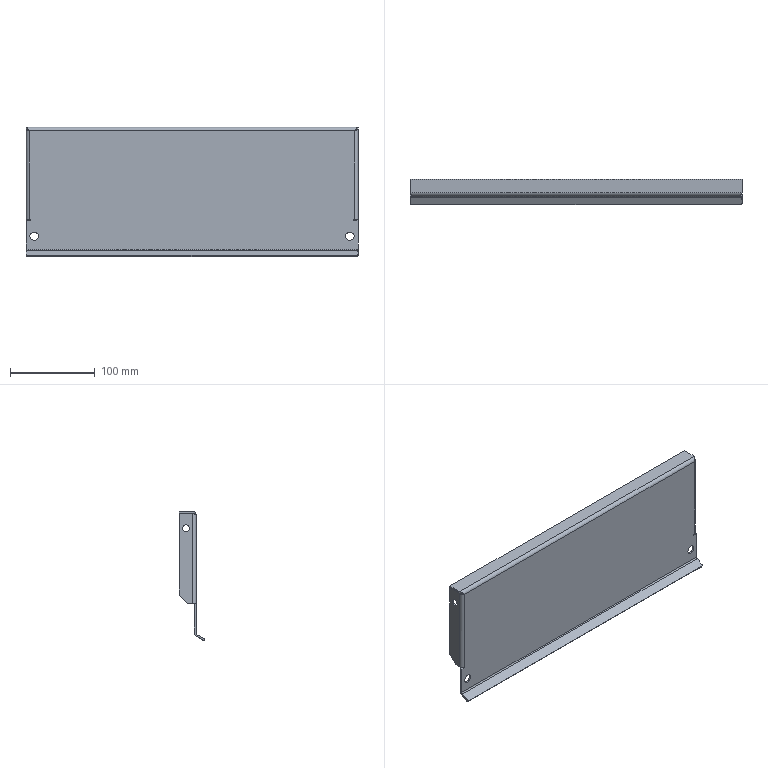Part | STEP file | SYL_0392D6J1SYL0380DJ100-571255 | 1 solid | 58 faces | box 392 x 30.392 x 152.732 mm | volume 143186 mm3 | plane 36 | cylinder 18 | spline 4 | commonest cylinder face diameters 8 x8 4 x6 10 x4